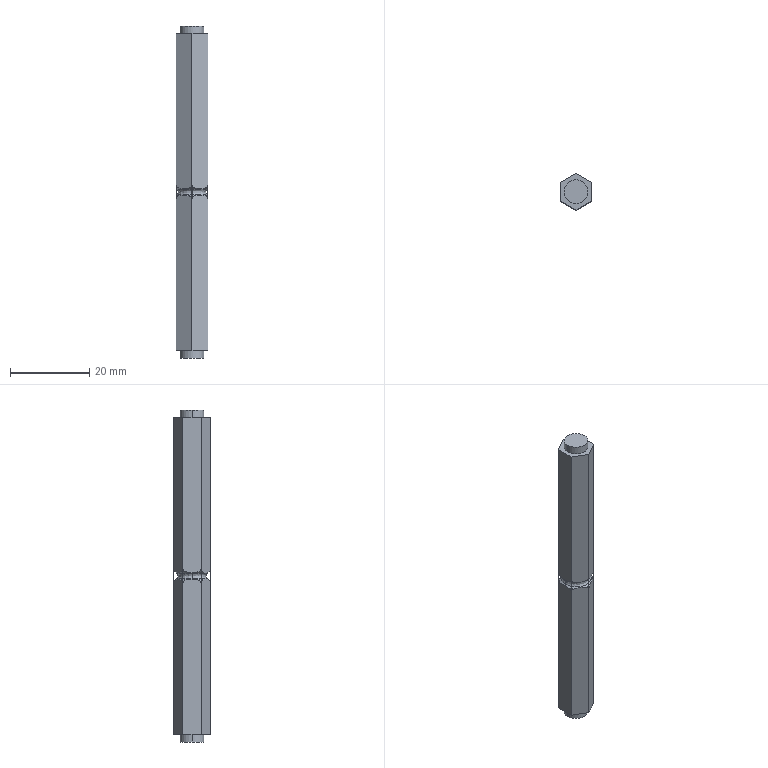Part | STEP file | 1 solid | 38 faces | box 8 x 9.238 x 84 mm | volume 4524 mm3 | spline 14 | cylinder 10 | plane 10 | cone 4 | commonest cylinder face diameters 9.214 x6 6 x4